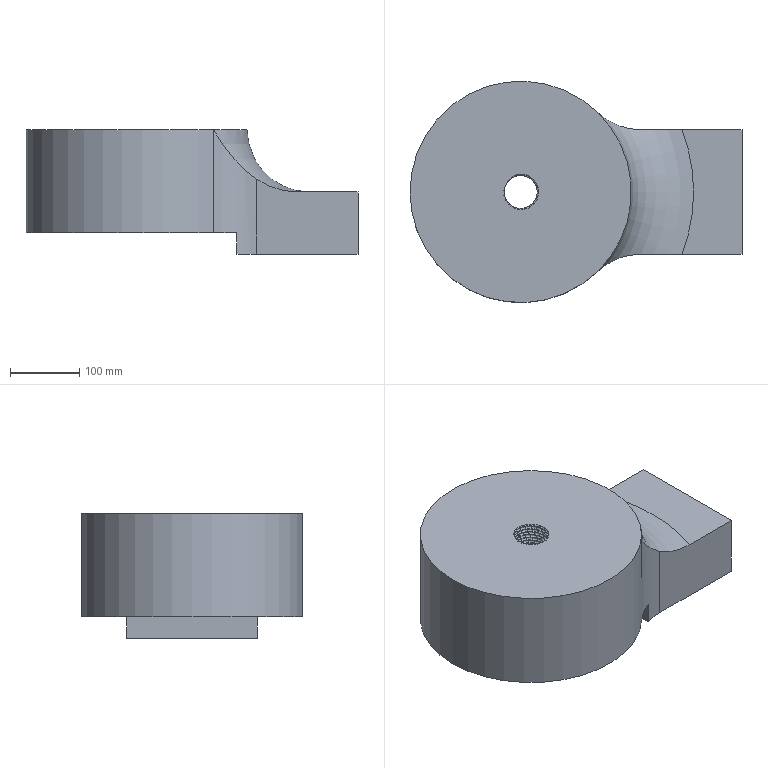Part | NX | features DATUM_CSYS 3, BLEND 2, CYLINDER 2, EXTRUDE 2, SKETCH 2, DATUM_PLANE 1, HELIX 1, SWP104 1 | 1 solid | 618 faces | box 480 x 320 x 180 mm | volume 14833518 mm3 | torus 606 | plane 8 | cylinder 4 | commonest cylinder face diameters 180 x2 48 x1 320 x1